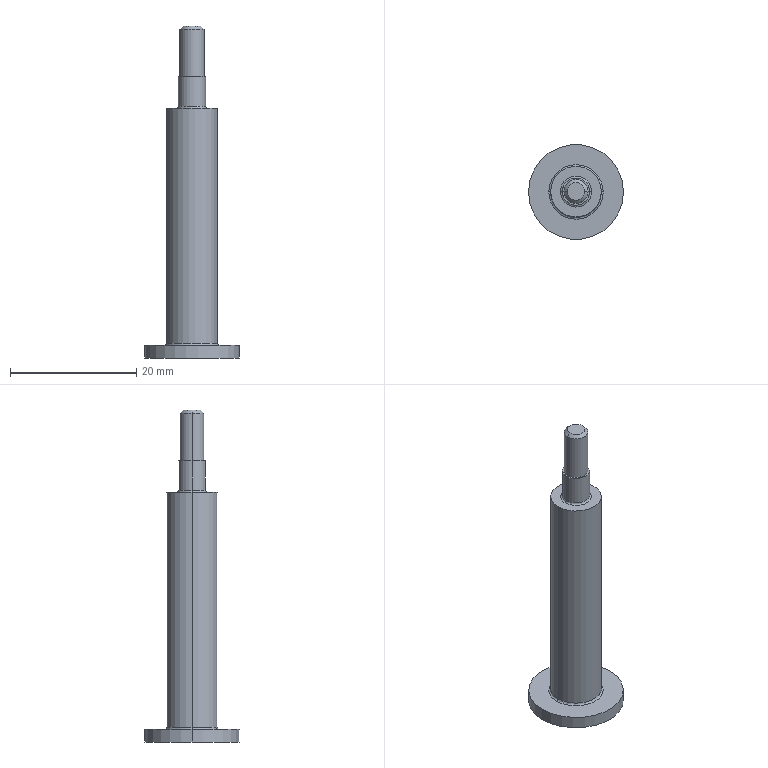Part | STEP file | Circlip check locating post-PN_0001 | 1 solid | 19 faces | box 15 x 15 x 52.5 mm | volume 2401 mm3 | cylinder 8 | plane 5 | spline 4 | cone 2 | commonest cylinder face diameters 3.8 x2 4.3 x2 8 x2 15 x2